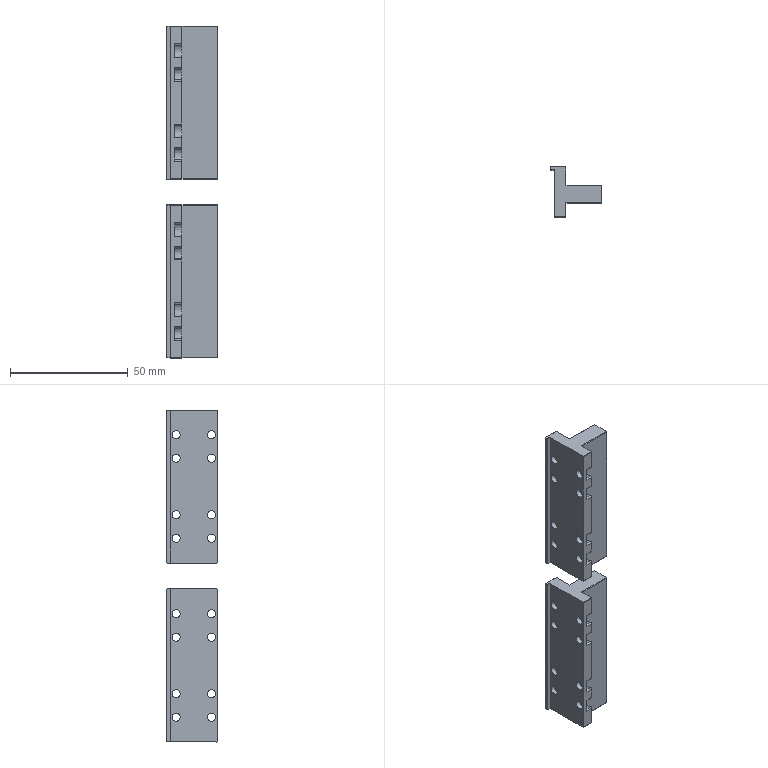Part | 2 solids | 118 faces | box 21.5 x 21.5 x 141 mm | volume 26725 mm3 | plane 64 | cylinder 54 | commonest cylinder face diameters 1 x16 3.5 x16 6 x16 3.3 x6